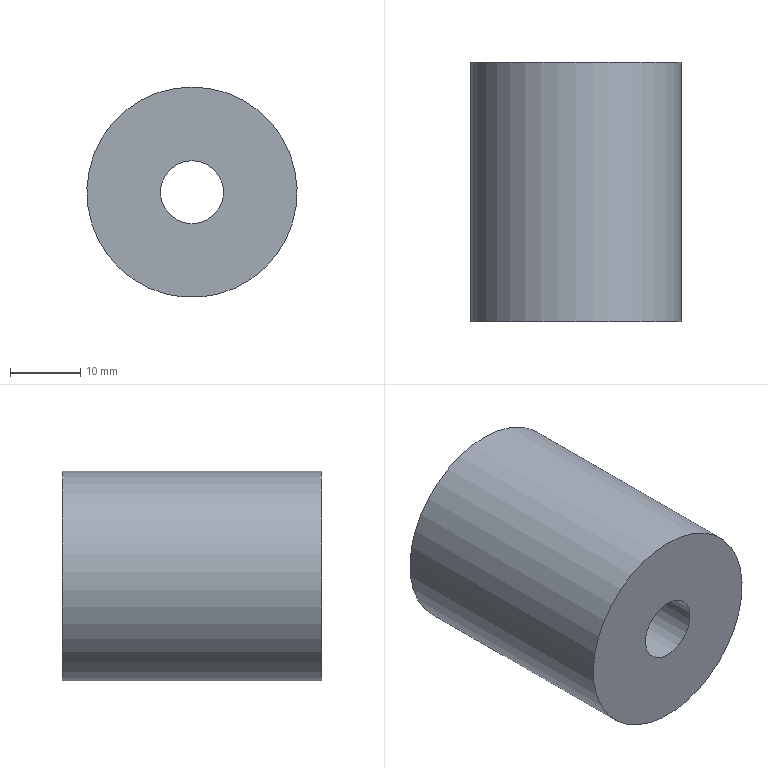Part | STEP file | DECH02 | 1 solid | 4 faces | box 30 x 37 x 30 mm | volume 23800 mm3 | plane 2 | cylinder 2 | commonest cylinder face diameters 9 x1 30 x1
STEP:
#1=CARTESIAN_POINT('',(0.,0.,0.));
#2=DIRECTION('',(0.,0.,1.));
#3=DIRECTION('',(1.,0.,0.));
#4=AXIS2_PLACEMENT_3D('',#1,#2,#3);
#5=CARTESIAN_POINT('',(0.,37.,15.));
#6=VERTEX_POINT('',#5);
#7=CARTESIAN_POINT('',(0.,37.,0.));
#8=DIRECTION('',(0.,1.,0.));
#9=DIRECTION('',(0.,0.,1.));
#10=AXIS2_PLACEMENT_3D('',#7,#8,#9);
#11=CIRCLE('',#10,15.);
#12=CARTESIAN_POINT('',(0.,37.,0.));
#13=DIRECTION('',(0.,1.,0.));
#14=DIRECTION('',(0.,0.,1.));
#15=AXIS2_PLACEMENT_3D('',#12,#13,#14);
#16=PLANE('',#15);
#17=CARTESIAN_POINT('',(0.,0.));
#18=DIRECTION('',(1.,0.));
#19=AXIS2_PLACEMENT_2D('',#17,#18);
#20=CIRCLE('',#19,15.);
#21=(GEOMETRIC_REPRESENTATION_CONTEXT(2)PARAMETRIC_REPRESENTATION_CONTEXT()REPRESENTATION_CONTEXT('',''));
#22=DEFINITIONAL_REPRESENTATION('',(#20),#21);
#23=PCURVE('',#16,#22);
#24=CARTESIAN_POINT('',(0.,37.,0.));
#25=DIRECTION('',(0.,-1.,0.));
#26=DIRECTION('',(0.,0.,-1.));
#27=AXIS2_PLACEMENT_3D('',#24,#25,#26);
#28=CYLINDRICAL_SURFACE('',#27,15.);
#29=CARTESIAN_POINT('',(9.425,0.));
#30=DIRECTION('',(-1.,0.));
#31=VECTOR('',#30,1.);
#32=LINE('',#29,#31);
#33=(GEOMETRIC_REPRESENTATION_CONTEXT(2)PARAMETRIC_REPRESENTATION_CONTEXT()REPRESENTATION_CONTEXT('',''));
#34=DEFINITIONAL_REPRESENTATION('',(#32),#33);
#35=PCURVE('',#28,#34);
#36=SURFACE_CURVE('',#11,(#23,#35),.PCURVE_S1.);
#37=EDGE_CURVE('',#6,#6,#36,.T.);
#38=ORIENTED_EDGE('',*,*,#37,.T.);
#39=EDGE_LOOP('',(#38));
#40=FACE_BOUND('',#39,.T.);
#41=CARTESIAN_POINT('',(0.,37.,4.5));
#42=VERTEX_POINT('',#41);
#43=CARTESIAN_POINT('',(0.,37.,0.));
#44=DIRECTION('',(0.,1.,0.));
#45=DIRECTION('',(0.,0.,1.));
#46=AXIS2_PLACEMENT_3D('',#43,#44,#45);
#47=CIRCLE('',#46,4.5);
#48=CARTESIAN_POINT('',(0.,0.));
#49=DIRECTION('',(1.,0.));
#50=AXIS2_PLACEMENT_2D('',#48,#49);
#51=CIRCLE('',#50,4.5);
#52=(GEOMETRIC_REPRESENTATION_CONTEXT(2)PARAMETRIC_REPRESENTATION_CONTEXT()REPRESENTATION_CONTEXT('',''));
#53=DEFINITIONAL_REPRESENTATION('',(#51),#52);
#54=PCURVE('',#16,#53);
#55=CARTESIAN_POINT('',(0.,37.,0.));
#56=DIRECTION('',(0.,-1.,0.));
#57=DIRECTION('',(0.,0.,-1.));
#58=AXIS2_PLACEMENT_3D('',#55,#56,#57);
#59=CYLINDRICAL_SURFACE('',#58,4.5);
#60=CARTESIAN_POINT('',(9.425,0.));
#61=DIRECTION('',(-1.,0.));
#62=VECTOR('',#61,1.);
#63=LINE('',#60,#62);
#64=(GEOMETRIC_REPRESENTATION_CONTEXT(2)PARAMETRIC_REPRESENTATION_CONTEXT()REPRESENTATION_CONTEXT('',''));
#65=DEFINITIONAL_REPRESENTATION('',(#63),#64);
#66=PCURVE('',#59,#65);
#67=SURFACE_CURVE('',#47,(#54,#66),.PCURVE_S1.);
#68=EDGE_CURVE('',#42,#42,#67,.T.);
#69=ORIENTED_EDGE('',*,*,#68,.F.);
#70=EDGE_LOOP('',(#69));
#71=FACE_BOUND('',#70,.T.);
#72=ADVANCED_FACE('',(#40,#71),#16,.T.);
#73=CARTESIAN_POINT('',(0.,0.,15.));
#74=VERTEX_POINT('',#73);
#75=CARTESIAN_POINT('',(0.,0.,0.));
#76=DIRECTION('',(0.,1.,0.));
#77=DIRECTION('',(0.,0.,1.));
#78=AXIS2_PLACEMENT_3D('',#75,#76,#77);
#79=CIRCLE('',#78,15.);
#80=CARTESIAN_POINT('',(0.,0.,0.));
#81=DIRECTION('',(0.,1.,0.));
#82=DIRECTION('',(0.,0.,1.));
#83=AXIS2_PLACEMENT_3D('',#80,#81,#82);
#84=PLANE('',#83);
#85=CARTESIAN_POINT('',(0.,0.));
#86=DIRECTION('',(1.,0.));
#87=AXIS2_PLACEMENT_2D('',#85,#86);
#88=CIRCLE('',#87,15.);
#89=(GEOMETRIC_REPRESENTATION_CONTEXT(2)PARAMETRIC_REPRESENTATION_CONTEXT()REPRESENTATION_CONTEXT('',''));
#90=DEFINITIONAL_REPRESENTATION('',(#88),#89);
#91=PCURVE('',#84,#90);
#92=CARTESIAN_POINT('',(9.425,37.));
#93=DIRECTION('',(-1.,0.));
#94=VECTOR('',#93,1.);
#95=LINE('',#92,#94);
#96=(GEOMETRIC_REPRESENTATION_CONTEXT(2)PARAMETRIC_REPRESENTATION_CONTEXT()REPRESENTATION_CONTEXT('',''));
#97=DEFINITIONAL_REPRESENTATION('',(#95),#96);
#98=PCURVE('',#28,#97);
#99=SURFACE_CURVE('',#79,(#91,#98),.PCURVE_S1.);
#100=EDGE_CURVE('',#74,#74,#99,.T.);
#101=ORIENTED_EDGE('',*,*,#100,.F.);
#102=EDGE_LOOP('',(#101));
#103=FACE_BOUND('',#102,.T.);
#104=CARTESIAN_POINT('',(0.,0.,4.5));
#105=VERTEX_POINT('',#104);
#106=CARTESIAN_POINT('',(0.,0.,0.));
#107=DIRECTION('',(0.,1.,0.));
#108=DIRECTION('',(0.,0.,1.));
#109=AXIS2_PLACEMENT_3D('',#106,#107,#108);
#110=CIRCLE('',#109,4.5);
#111=CARTESIAN_POINT('',(0.,0.));
#112=DIRECTION('',(1.,0.));
#113=AXIS2_PLACEMENT_2D('',#111,#112);
#114=CIRCLE('',#113,4.5);
#115=(GEOMETRIC_REPRESENTATION_CONTEXT(2)PARAMETRIC_REPRESENTATION_CONTEXT()REPRESENTATION_CONTEXT('',''));
#116=DEFINITIONAL_REPRESENTATION('',(#114),#115);
#117=PCURVE('',#84,#116);
#118=CARTESIAN_POINT('',(9.425,37.));
#119=DIRECTION('',(-1.,0.));
#120=VECTOR('',#119,1.);
#121=LINE('',#118,#120);
#122=(GEOMETRIC_REPRESENTATION_CONTEXT(2)PARAMETRIC_REPRESENTATION_CONTEXT()REPRESENTATION_CONTEXT('',''));
#123=DEFINITIONAL_REPRESENTATION('',(#121),#122);
#124=PCURVE('',#59,#123);
#125=SURFACE_CURVE('',#110,(#117,#124),.PCURVE_S1.);
#126=EDGE_CURVE('',#105,#105,#125,.T.);
#127=ORIENTED_EDGE('',*,*,#126,.T.);
#128=EDGE_LOOP('',(#127));
#129=FACE_BOUND('',#128,.T.);
#130=ADVANCED_FACE('',(#103,#129),#84,.F.);
#131=ORIENTED_EDGE('',*,*,#37,.F.);
#132=CARTESIAN_POINT('',(0.,37.,15.));
#133=CARTESIAN_POINT('',(0.,0.,15.));
#134=B_SPLINE_CURVE_WITH_KNOTS('',1,(#132,#133),.UNSPECIFIED.,.F.,.F.,(2,2),(0.,37.),.PIECEWISE_BEZIER_KNOTS.);
#135=CARTESIAN_POINT('',(9.425,0.));
#136=DIRECTION('',(0.,1.));
#137=VECTOR('',#136,1.);
#138=LINE('',#135,#137);
#139=(GEOMETRIC_REPRESENTATION_CONTEXT(2)PARAMETRIC_REPRESENTATION_CONTEXT()REPRESENTATION_CONTEXT('',''));
#140=DEFINITIONAL_REPRESENTATION('',(#138),#139);
#141=PCURVE('',#28,#140);
#142=CARTESIAN_POINT('',(3.142,0.));
#143=DIRECTION('',(0.,1.));
#144=VECTOR('',#143,1.);
#145=LINE('',#142,#144);
#146=(GEOMETRIC_REPRESENTATION_CONTEXT(2)PARAMETRIC_REPRESENTATION_CONTEXT()REPRESENTATION_CONTEXT('',''));
#147=DEFINITIONAL_REPRESENTATION('',(#145),#146);
#148=PCURVE('',#28,#147);
#149=SEAM_CURVE('',#134,(#141,#148),.PCURVE_S1.);
#150=EDGE_CURVE('',#6,#74,#149,.T.);
#151=ORIENTED_EDGE('',*,*,#150,.T.);
#152=ORIENTED_EDGE('',*,*,#100,.T.);
#153=ORIENTED_EDGE('',*,*,#150,.F.);
#154=EDGE_LOOP('',(#131,#151,#152,#153));
#155=FACE_BOUND('',#154,.T.);
#156=ADVANCED_FACE('',(#155),#28,.T.);
#157=ORIENTED_EDGE('',*,*,#68,.F.);
#158=CARTESIAN_POINT('',(0.,37.,4.5));
#159=CARTESIAN_POINT('',(0.,0.,4.5));
#160=B_SPLINE_CURVE_WITH_KNOTS('',1,(#158,#159),.UNSPECIFIED.,.F.,.F.,(2,2),(0.,37.),.PIECEWISE_BEZIER_KNOTS.);
#161=CARTESIAN_POINT('',(9.425,0.));
#162=DIRECTION('',(0.,1.));
#163=VECTOR('',#162,1.);
#164=LINE('',#161,#163);
#165=(GEOMETRIC_REPRESENTATION_CONTEXT(2)PARAMETRIC_REPRESENTATION_CONTEXT()REPRESENTATION_CONTEXT('',''));
#166=DEFINITIONAL_REPRESENTATION('',(#164),#165);
#167=PCURVE('',#59,#166);
#168=CARTESIAN_POINT('',(3.142,0.));
#169=DIRECTION('',(0.,1.));
#170=VECTOR('',#169,1.);
#171=LINE('',#168,#170);
#172=(GEOMETRIC_REPRESENTATION_CONTEXT(2)PARAMETRIC_REPRESENTATION_CONTEXT()REPRESENTATION_CONTEXT('',''));
#173=DEFINITIONAL_REPRESENTATION('',(#171),#172);
#174=PCURVE('',#59,#173);
#175=SEAM_CURVE('',#160,(#167,#174),.PCURVE_S1.);
#176=EDGE_CURVE('',#42,#105,#175,.T.);
#177=ORIENTED_EDGE('',*,*,#176,.T.);
#178=ORIENTED_EDGE('',*,*,#126,.T.);
#179=ORIENTED_EDGE('',*,*,#176,.F.);
#180=EDGE_LOOP('',(#157,#177,#178,#179));
#181=FACE_BOUND('',#180,.F.);
#182=ADVANCED_FACE('',(#181),#59,.F.);
#183=CLOSED_SHELL('',(#72,#130,#156,#182));
#184=MANIFOLD_SOLID_BREP('',#183);
#185=(LENGTH_UNIT()NAMED_UNIT(*)SI_UNIT(.MILLI.,.METRE.));
#186=UNCERTAINTY_MEASURE_WITH_UNIT(LENGTH_MEASURE(0.00001),#185,'','');
#187=(NAMED_UNIT(*)PLANE_ANGLE_UNIT()SI_UNIT($,.RADIAN.));
#188=(NAMED_UNIT(*)SI_UNIT($,.STERADIAN.)SOLID_ANGLE_UNIT());
#189=(GEOMETRIC_REPRESENTATION_CONTEXT(3)GLOBAL_UNCERTAINTY_ASSIGNED_CONTEXT((#186))GLOBAL_UNIT_ASSIGNED_CONTEXT((#185,#187,#188))REPRESENTATION_CONTEXT('',''));
#190=ADVANCED_BREP_SHAPE_REPRESENTATION('',(#4,#184),#189);